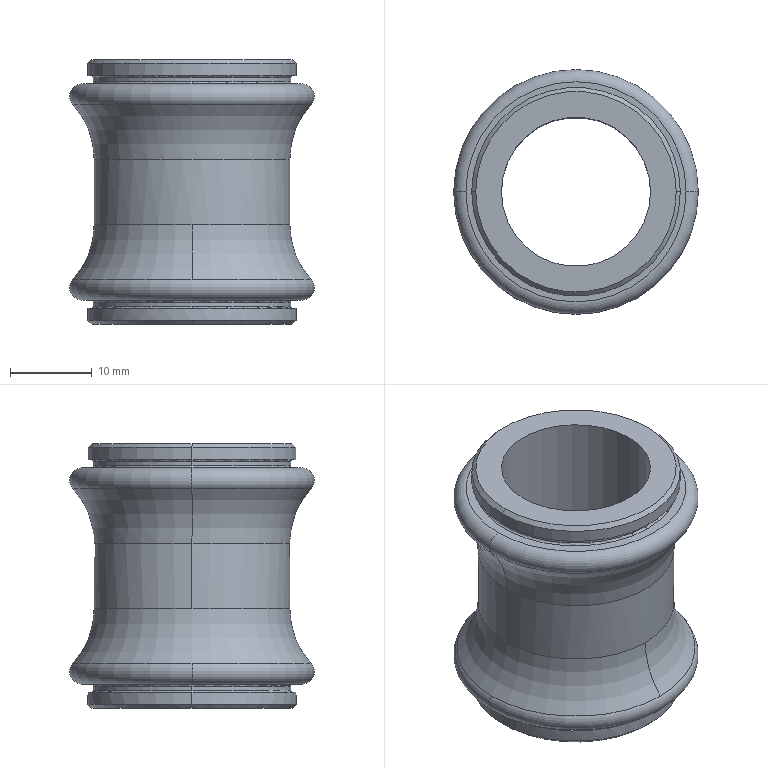Part | STEP file | _HSV08 -slide.... | 1 solid | 38 faces | box 30 x 30 x 32.5 mm | volume 8453 mm3 | torus 16 | cylinder 12 | plane 6 | cone 4 | commonest cylinder face diameters 24.2 x4 25.6 x4 18.3 x2 24 x2
STEP:
#1=CARTESIAN_POINT('',(-9.15,0.,0.));
#2=VERTEX_POINT('',#1);
#3=CARTESIAN_POINT('',(9.15,0.,0.));
#4=VERTEX_POINT('',#3);
#5=CARTESIAN_POINT('',(0.,0.,0.));
#6=DIRECTION('',(0.,0.,1.));
#7=DIRECTION('',(1.,0.,0.));
#8=AXIS2_PLACEMENT_3D('',#5,#6,#7);
#9=CIRCLE('',#8,9.15);
#10=EDGE_CURVE('',#2,#4,#9,.T.);
#11=ORIENTED_EDGE('',*,*,#10,.F.);
#12=CARTESIAN_POINT('',(-9.15,0.,32.5));
#13=VERTEX_POINT('',#12);
#14=CARTESIAN_POINT('',(-9.15,0.,0.));
#15=DIRECTION('',(0.,0.,1.));
#16=VECTOR('',#15,1000.);
#17=LINE('',#14,#16);
#18=EDGE_CURVE('',#2,#13,#17,.T.);
#19=ORIENTED_EDGE('',*,*,#18,.T.);
#20=CARTESIAN_POINT('',(9.15,0.,32.5));
#21=VERTEX_POINT('',#20);
#22=CARTESIAN_POINT('',(0.,0.,32.5));
#23=DIRECTION('',(0.,0.,-1.));
#24=DIRECTION('',(1.,0.,0.));
#25=AXIS2_PLACEMENT_3D('',#22,#23,#24);
#26=CIRCLE('',#25,9.15);
#27=EDGE_CURVE('',#21,#13,#26,.T.);
#28=ORIENTED_EDGE('',*,*,#27,.F.);
#29=CARTESIAN_POINT('',(9.15,0.,0.));
#30=DIRECTION('',(0.,0.,1.));
#31=VECTOR('',#30,1000.);
#32=LINE('',#29,#31);
#33=EDGE_CURVE('',#4,#21,#32,.T.);
#34=ORIENTED_EDGE('',*,*,#33,.F.);
#35=EDGE_LOOP('',(#11,#19,#28,#34));
#36=FACE_OUTER_BOUND('',#35,.T.);
#37=CARTESIAN_POINT('',(0.,0.,0.));
#38=DIRECTION('',(0.,0.,1.));
#39=DIRECTION('',(1.,0.,0.));
#40=AXIS2_PLACEMENT_3D('',#37,#38,#39);
#41=CYLINDRICAL_SURFACE('',#40,9.15);
#42=ADVANCED_FACE('',(#36),#41,.F.);
#43=CARTESIAN_POINT('',(0.,12.3,0.));
#44=VERTEX_POINT('',#43);
#45=CARTESIAN_POINT('',(0.,-12.3,0.));
#46=VERTEX_POINT('',#45);
#47=CARTESIAN_POINT('',(0.,0.,0.));
#48=DIRECTION('',(0.,0.,-1.));
#49=DIRECTION('',(0.,-1.,0.));
#50=AXIS2_PLACEMENT_3D('',#47,#48,#49);
#51=CIRCLE('',#50,12.3);
#52=EDGE_CURVE('',#44,#46,#51,.T.);
#53=ORIENTED_EDGE('',*,*,#52,.F.);
#54=CARTESIAN_POINT('',(0.,12.8,0.5));
#55=VERTEX_POINT('',#54);
#56=CARTESIAN_POINT('',(0.,12.8,0.5));
#57=DIRECTION('',(0.,0.7071,0.7071));
#58=VECTOR('',#57,1000.);
#59=LINE('',#56,#58);
#60=EDGE_CURVE('',#44,#55,#59,.T.);
#61=ORIENTED_EDGE('',*,*,#60,.T.);
#62=CARTESIAN_POINT('',(12.8,0.,0.5));
#63=VERTEX_POINT('',#62);
#64=CARTESIAN_POINT('',(0.,0.,0.5));
#65=DIRECTION('',(0.,0.,-1.));
#66=DIRECTION('',(1.,0.,0.));
#67=AXIS2_PLACEMENT_3D('',#64,#65,#66);
#68=CIRCLE('',#67,12.8);
#69=EDGE_CURVE('',#55,#63,#68,.T.);
#70=ORIENTED_EDGE('',*,*,#69,.T.);
#71=CARTESIAN_POINT('',(0.,-12.8,0.5));
#72=VERTEX_POINT('',#71);
#73=CARTESIAN_POINT('',(0.,0.,0.5));
#74=DIRECTION('',(0.,0.,-1.));
#75=DIRECTION('',(1.,0.,0.));
#76=AXIS2_PLACEMENT_3D('',#73,#74,#75);
#77=CIRCLE('',#76,12.8);
#78=EDGE_CURVE('',#63,#72,#77,.T.);
#79=ORIENTED_EDGE('',*,*,#78,.T.);
#80=CARTESIAN_POINT('',(0.,-12.8,0.5));
#81=DIRECTION('',(0.,-0.7071,0.7071));
#82=VECTOR('',#81,1000.);
#83=LINE('',#80,#82);
#84=EDGE_CURVE('',#46,#72,#83,.T.);
#85=ORIENTED_EDGE('',*,*,#84,.F.);
#86=EDGE_LOOP('',(#53,#61,#70,#79,#85));
#87=FACE_OUTER_BOUND('',#86,.T.);
#88=CARTESIAN_POINT('',(0.,0.,0.5));
#89=DIRECTION('',(0.,0.,1.));
#90=DIRECTION('',(0.,-1.,0.));
#91=AXIS2_PLACEMENT_3D('',#88,#89,#90);
#92=CONICAL_SURFACE('',#91,12.8,0.7854);
#93=ADVANCED_FACE('',(#87),#92,.T.);
#94=CARTESIAN_POINT('',(12.3,0.,32.5));
#95=VERTEX_POINT('',#94);
#96=CARTESIAN_POINT('',(-12.3,0.,32.5));
#97=VERTEX_POINT('',#96);
#98=CARTESIAN_POINT('',(0.,0.,32.5));
#99=DIRECTION('',(0.,0.,1.));
#100=DIRECTION('',(-1.,0.,0.));
#101=AXIS2_PLACEMENT_3D('',#98,#99,#100);
#102=CIRCLE('',#101,12.3);
#103=EDGE_CURVE('',#95,#97,#102,.T.);
#104=ORIENTED_EDGE('',*,*,#103,.F.);
#105=CARTESIAN_POINT('',(12.8,0.,32.));
#106=VERTEX_POINT('',#105);
#107=CARTESIAN_POINT('',(12.8,0.,32.));
#108=DIRECTION('',(0.7071,0.,-0.7071));
#109=VECTOR('',#108,1000.);
#110=LINE('',#107,#109);
#111=EDGE_CURVE('',#95,#106,#110,.T.);
#112=ORIENTED_EDGE('',*,*,#111,.T.);
#113=CARTESIAN_POINT('',(-12.8,0.,32.));
#114=VERTEX_POINT('',#113);
#115=CARTESIAN_POINT('',(0.,0.,32.));
#116=DIRECTION('',(0.,0.,1.));
#117=DIRECTION('',(-1.,0.,0.));
#118=AXIS2_PLACEMENT_3D('',#115,#116,#117);
#119=CIRCLE('',#118,12.8);
#120=EDGE_CURVE('',#106,#114,#119,.T.);
#121=ORIENTED_EDGE('',*,*,#120,.T.);
#122=CARTESIAN_POINT('',(-12.8,0.,32.));
#123=DIRECTION('',(-0.7071,0.,-0.7071));
#124=VECTOR('',#123,1000.);
#125=LINE('',#122,#124);
#126=EDGE_CURVE('',#97,#114,#125,.T.);
#127=ORIENTED_EDGE('',*,*,#126,.F.);
#128=EDGE_LOOP('',(#104,#112,#121,#127));
#129=FACE_OUTER_BOUND('',#128,.T.);
#130=CARTESIAN_POINT('',(0.,0.,32.));
#131=DIRECTION('',(0.,0.,-1.));
#132=DIRECTION('',(-1.,0.,0.));
#133=AXIS2_PLACEMENT_3D('',#130,#131,#132);
#134=CONICAL_SURFACE('',#133,12.8,0.7854);
#135=ADVANCED_FACE('',(#129),#134,.T.);
#136=CARTESIAN_POINT('',(-12.8,0.,0.5));
#137=VERTEX_POINT('',#136);
#138=CARTESIAN_POINT('',(0.,0.,0.5));
#139=DIRECTION('',(0.,0.,-1.));
#140=DIRECTION('',(1.,0.,0.));
#141=AXIS2_PLACEMENT_3D('',#138,#139,#140);
#142=CIRCLE('',#141,12.8);
#143=EDGE_CURVE('',#137,#55,#142,.T.);
#144=ORIENTED_EDGE('',*,*,#143,.F.);
#145=CARTESIAN_POINT('',(-12.8,0.,2.));
#146=VERTEX_POINT('',#145);
#147=CARTESIAN_POINT('',(-12.8,0.,0.));
#148=DIRECTION('',(0.,0.,1.));
#149=VECTOR('',#148,1000.);
#150=LINE('',#147,#149);
#151=EDGE_CURVE('',#137,#146,#150,.T.);
#152=ORIENTED_EDGE('',*,*,#151,.T.);
#153=CARTESIAN_POINT('',(12.8,0.,2.));
#154=VERTEX_POINT('',#153);
#155=CARTESIAN_POINT('',(0.,0.,2.));
#156=DIRECTION('',(0.,0.,-1.));
#157=DIRECTION('',(1.,0.,0.));
#158=AXIS2_PLACEMENT_3D('',#155,#156,#157);
#159=CIRCLE('',#158,12.8);
#160=EDGE_CURVE('',#146,#154,#159,.T.);
#161=ORIENTED_EDGE('',*,*,#160,.T.);
#162=CARTESIAN_POINT('',(12.8,0.,0.));
#163=DIRECTION('',(0.,0.,1.));
#164=VECTOR('',#163,1000.);
#165=LINE('',#162,#164);
#166=EDGE_CURVE('',#63,#154,#165,.T.);
#167=ORIENTED_EDGE('',*,*,#166,.F.);
#168=ORIENTED_EDGE('',*,*,#69,.F.);
#169=EDGE_LOOP('',(#144,#152,#161,#167,#168));
#170=FACE_OUTER_BOUND('',#169,.T.);
#171=CARTESIAN_POINT('',(0.,0.,0.));
#172=DIRECTION('',(0.,0.,1.));
#173=DIRECTION('',(1.,0.,0.));
#174=AXIS2_PLACEMENT_3D('',#171,#172,#173);
#175=CYLINDRICAL_SURFACE('',#174,12.8);
#176=ADVANCED_FACE('',(#170),#175,.T.);
#177=CARTESIAN_POINT('',(12.8,0.,30.5));
#178=VERTEX_POINT('',#177);
#179=CARTESIAN_POINT('',(-12.8,0.,30.5));
#180=VERTEX_POINT('',#179);
#181=CARTESIAN_POINT('',(0.,0.,30.5));
#182=DIRECTION('',(0.,0.,1.));
#183=DIRECTION('',(1.,0.,0.));
#184=AXIS2_PLACEMENT_3D('',#181,#182,#183);
#185=CIRCLE('',#184,12.8);
#186=EDGE_CURVE('',#178,#180,#185,.T.);
#187=ORIENTED_EDGE('',*,*,#186,.T.);
#188=CARTESIAN_POINT('',(-12.8,0.,0.));
#189=DIRECTION('',(0.,0.,1.));
#190=VECTOR('',#189,1000.);
#191=LINE('',#188,#190);
#192=EDGE_CURVE('',#180,#114,#191,.T.);
#193=ORIENTED_EDGE('',*,*,#192,.T.);
#194=ORIENTED_EDGE('',*,*,#120,.F.);
#195=CARTESIAN_POINT('',(12.8,0.,0.));
#196=DIRECTION('',(0.,0.,1.));
#197=VECTOR('',#196,1000.);
#198=LINE('',#195,#197);
#199=EDGE_CURVE('',#178,#106,#198,.T.);
#200=ORIENTED_EDGE('',*,*,#199,.F.);
#201=EDGE_LOOP('',(#187,#193,#194,#200));
#202=FACE_OUTER_BOUND('',#201,.T.);
#203=CARTESIAN_POINT('',(0.,0.,0.));
#204=DIRECTION('',(0.,0.,1.));
#205=DIRECTION('',(1.,0.,0.));
#206=AXIS2_PLACEMENT_3D('',#203,#204,#205);
#207=CYLINDRICAL_SURFACE('',#206,12.8);
#208=ADVANCED_FACE('',(#202),#207,.T.);
#209=CARTESIAN_POINT('',(0.,-12.35,2.));
#210=VERTEX_POINT('',#209);
#211=CARTESIAN_POINT('',(0.,12.35,2.));
#212=VERTEX_POINT('',#211);
#213=CARTESIAN_POINT('',(0.,0.,2.));
#214=DIRECTION('',(0.,0.,-1.));
#215=DIRECTION('',(0.,1.,0.));
#216=AXIS2_PLACEMENT_3D('',#213,#214,#215);
#217=CIRCLE('',#216,12.35);
#218=EDGE_CURVE('',#210,#212,#217,.T.);
#219=ORIENTED_EDGE('',*,*,#218,.F.);
#220=CARTESIAN_POINT('',(0.,-12.1,2.25));
#221=VERTEX_POINT('',#220);
#222=CARTESIAN_POINT('',(0.,-12.35,2.25));
#223=DIRECTION('',(1.,0.,0.));
#224=DIRECTION('',(0.,1.,0.));
#225=AXIS2_PLACEMENT_3D('',#222,#223,#224);
#226=CIRCLE('',#225,0.25);
#227=EDGE_CURVE('',#210,#221,#226,.T.);
#228=ORIENTED_EDGE('',*,*,#227,.T.);
#229=CARTESIAN_POINT('',(-12.1,0.,2.25));
#230=VERTEX_POINT('',#229);
#231=CARTESIAN_POINT('',(0.,0.,2.25));
#232=DIRECTION('',(0.,0.,1.));
#233=DIRECTION('',(1.,0.,0.));
#234=AXIS2_PLACEMENT_3D('',#231,#232,#233);
#235=CIRCLE('',#234,12.1);
#236=EDGE_CURVE('',#230,#221,#235,.T.);
#237=ORIENTED_EDGE('',*,*,#236,.F.);
#238=CARTESIAN_POINT('',(0.,12.1,2.25));
#239=VERTEX_POINT('',#238);
#240=CARTESIAN_POINT('',(0.,0.,2.25));
#241=DIRECTION('',(0.,0.,1.));
#242=DIRECTION('',(1.,0.,0.));
#243=AXIS2_PLACEMENT_3D('',#240,#241,#242);
#244=CIRCLE('',#243,12.1);
#245=EDGE_CURVE('',#239,#230,#244,.T.);
#246=ORIENTED_EDGE('',*,*,#245,.F.);
#247=CARTESIAN_POINT('',(0.,12.35,2.25));
#248=DIRECTION('',(-1.,0.,0.));
#249=DIRECTION('',(0.,0.,1.));
#250=AXIS2_PLACEMENT_3D('',#247,#248,#249);
#251=CIRCLE('',#250,0.25);
#252=EDGE_CURVE('',#212,#239,#251,.T.);
#253=ORIENTED_EDGE('',*,*,#252,.F.);
#254=EDGE_LOOP('',(#219,#228,#237,#246,#253));
#255=FACE_OUTER_BOUND('',#254,.T.);
#256=CARTESIAN_POINT('',(0.,0.,2.25));
#257=DIRECTION('',(0.,0.,-1.));
#258=DIRECTION('',(0.,1.,0.));
#259=AXIS2_PLACEMENT_3D('',#256,#257,#258);
#260=TOROIDAL_SURFACE('',#259,12.35,0.25);
#261=ADVANCED_FACE('',(#255),#260,.F.);
#262=CARTESIAN_POINT('',(0.,-12.1,30.25));
#263=VERTEX_POINT('',#262);
#264=CARTESIAN_POINT('',(-12.1,0.,30.25));
#265=VERTEX_POINT('',#264);
#266=CARTESIAN_POINT('',(0.,0.,30.25));
#267=DIRECTION('',(0.,0.,-1.));
#268=DIRECTION('',(-1.,0.,0.));
#269=AXIS2_PLACEMENT_3D('',#266,#267,#268);
#270=CIRCLE('',#269,12.1);
#271=EDGE_CURVE('',#263,#265,#270,.T.);
#272=ORIENTED_EDGE('',*,*,#271,.F.);
#273=CARTESIAN_POINT('',(0.,-12.35,30.5));
#274=VERTEX_POINT('',#273);
#275=CARTESIAN_POINT('',(0.,-12.35,30.25));
#276=DIRECTION('',(1.,0.,0.));
#277=DIRECTION('',(0.,1.,0.));
#278=AXIS2_PLACEMENT_3D('',#275,#276,#277);
#279=CIRCLE('',#278,0.25);
#280=EDGE_CURVE('',#263,#274,#279,.T.);
#281=ORIENTED_EDGE('',*,*,#280,.T.);
#282=CARTESIAN_POINT('',(0.,12.35,30.5));
#283=VERTEX_POINT('',#282);
#284=CARTESIAN_POINT('',(0.,0.,30.5));
#285=DIRECTION('',(0.,0.,1.));
#286=DIRECTION('',(0.,1.,0.));
#287=AXIS2_PLACEMENT_3D('',#284,#285,#286);
#288=CIRCLE('',#287,12.35);
#289=EDGE_CURVE('',#283,#274,#288,.T.);
#290=ORIENTED_EDGE('',*,*,#289,.F.);
#291=CARTESIAN_POINT('',(0.,12.1,30.25));
#292=VERTEX_POINT('',#291);
#293=CARTESIAN_POINT('',(0.,12.35,30.25));
#294=DIRECTION('',(-1.,0.,0.));
#295=DIRECTION('',(0.,0.,1.));
#296=AXIS2_PLACEMENT_3D('',#293,#294,#295);
#297=CIRCLE('',#296,0.25);
#298=EDGE_CURVE('',#292,#283,#297,.T.);
#299=ORIENTED_EDGE('',*,*,#298,.F.);
#300=CARTESIAN_POINT('',(0.,0.,30.25));
#301=DIRECTION('',(0.,0.,-1.));
#302=DIRECTION('',(-1.,0.,0.));
#303=AXIS2_PLACEMENT_3D('',#300,#301,#302);
#304=CIRCLE('',#303,12.1);
#305=EDGE_CURVE('',#265,#292,#304,.T.);
#306=ORIENTED_EDGE('',*,*,#305,.F.);
#307=EDGE_LOOP('',(#272,#281,#290,#299,#306));
#308=FACE_OUTER_BOUND('',#307,.T.);
#309=CARTESIAN_POINT('',(0.,0.,30.25));
#310=DIRECTION('',(0.,0.,-1.));
#311=DIRECTION('',(0.,1.,0.));
#312=AXIS2_PLACEMENT_3D('',#309,#310,#311);
#313=TOROIDAL_SURFACE('',#312,12.35,0.25);
#314=ADVANCED_FACE('',(#308),#313,.F.);
#315=CARTESIAN_POINT('',(12.1,0.,2.25));
#316=VERTEX_POINT('',#315);
#317=CARTESIAN_POINT('',(0.,0.,2.25));
#318=DIRECTION('',(0.,0.,1.));
#319=DIRECTION('',(1.,0.,0.));
#320=AXIS2_PLACEMENT_3D('',#317,#318,#319);
#321=CIRCLE('',#320,12.1);
#322=EDGE_CURVE('',#316,#239,#321,.T.);
#323=ORIENTED_EDGE('',*,*,#322,.T.);
#324=ORIENTED_EDGE('',*,*,#245,.T.);
#325=CARTESIAN_POINT('',(-12.1,0.,2.75));
#326=VERTEX_POINT('',#325);
#327=CARTESIAN_POINT('',(-12.1,0.,0.));
#328=DIRECTION('',(0.,0.,1.));
#329=VECTOR('',#328,1000.);
#330=LINE('',#327,#329);
#331=EDGE_CURVE('',#230,#326,#330,.T.);
#332=ORIENTED_EDGE('',*,*,#331,.T.);
#333=CARTESIAN_POINT('',(0.,12.1,2.75));
#334=VERTEX_POINT('',#333);
#335=CARTESIAN_POINT('',(0.,0.,2.75));
#336=DIRECTION('',(0.,0.,-1.));
#337=DIRECTION('',(1.,0.,0.));
#338=AXIS2_PLACEMENT_3D('',#335,#336,#337);
#339=CIRCLE('',#338,12.1);
#340=EDGE_CURVE('',#326,#334,#339,.T.);
#341=ORIENTED_EDGE('',*,*,#340,.T.);
#342=CARTESIAN_POINT('',(12.1,0.,2.75));
#343=VERTEX_POINT('',#342);
#344=CARTESIAN_POINT('',(0.,0.,2.75));
#345=DIRECTION('',(0.,0.,-1.));
#346=DIRECTION('',(1.,0.,0.));
#347=AXIS2_PLACEMENT_3D('',#344,#345,#346);
#348=CIRCLE('',#347,12.1);
#349=EDGE_CURVE('',#334,#343,#348,.T.);
#350=ORIENTED_EDGE('',*,*,#349,.T.);
#351=CARTESIAN_POINT('',(12.1,0.,0.));
#352=DIRECTION('',(0.,0.,1.));
#353=VECTOR('',#352,1000.);
#354=LINE('',#351,#353);
#355=EDGE_CURVE('',#316,#343,#354,.T.);
#356=ORIENTED_EDGE('',*,*,#355,.F.);
#357=EDGE_LOOP('',(#323,#324,#332,#341,#350,#356));
#358=FACE_OUTER_BOUND('',#357,.T.);
#359=CARTESIAN_POINT('',(0.,0.,0.));
#360=DIRECTION('',(0.,0.,1.));
#361=DIRECTION('',(1.,0.,0.));
#362=AXIS2_PLACEMENT_3D('',#359,#360,#361);
#363=CYLINDRICAL_SURFACE('',#362,12.1);
#364=ADVANCED_FACE('',(#358),#363,.T.);
#365=CARTESIAN_POINT('',(0.,12.1,29.75));
#366=VERTEX_POINT('',#365);
#367=CARTESIAN_POINT('',(-12.1,0.,29.75));
#368=VERTEX_POINT('',#367);
#369=CARTESIAN_POINT('',(0.,0.,29.75));
#370=DIRECTION('',(0.,0.,1.));
#371=DIRECTION('',(1.,0.,0.));
#372=AXIS2_PLACEMENT_3D('',#369,#370,#371);
#373=CIRCLE('',#372,12.1);
#374=EDGE_CURVE('',#366,#368,#373,.T.);
#375=ORIENTED_EDGE('',*,*,#374,.T.);
#376=CARTESIAN_POINT('',(-12.1,0.,0.));
#377=DIRECTION('',(0.,0.,1.));
#378=VECTOR('',#377,1000.);
#379=LINE('',#376,#378);
#380=EDGE_CURVE('',#368,#265,#379,.T.);
#381=ORIENTED_EDGE('',*,*,#380,.T.);
#382=ORIENTED_EDGE('',*,*,#305,.T.);
#383=CARTESIAN_POINT('',(12.1,0.,30.25));
#384=VERTEX_POINT('',#383);
#385=CARTESIAN_POINT('',(0.,0.,30.25));
#386=DIRECTION('',(0.,0.,-1.));
#387=DIRECTION('',(-1.,0.,0.));
#388=AXIS2_PLACEMENT_3D('',#385,#386,#387);
#389=CIRCLE('',#388,12.1);
#390=EDGE_CURVE('',#292,#384,#389,.T.);
#391=ORIENTED_EDGE('',*,*,#390,.T.);
#392=CARTESIAN_POINT('',(12.1,0.,29.75));
#393=VERTEX_POINT('',#392);
#394=CARTESIAN_POINT('',(12.1,0.,0.));
#395=DIRECTION('',(0.,0.,1.));
#396=VECTOR('',#395,1000.);
#397=LINE('',#394,#396);
#398=EDGE_CURVE('',#393,#384,#397,.T.);
#399=ORIENTED_EDGE('',*,*,#398,.F.);
#400=CARTESIAN_POINT('',(0.,0.,29.75));
#401=DIRECTION('',(0.,0.,1.));
#402=DIRECTION('',(1.,0.,0.));
#403=AXIS2_PLACEMENT_3D('',#400,#401,#402);
#404=CIRCLE('',#403,12.1);
#405=EDGE_CURVE('',#393,#366,#404,.T.);
#406=ORIENTED_EDGE('',*,*,#405,.T.);
#407=EDGE_LOOP('',(#375,#381,#382,#391,#399,#406));
#408=FACE_OUTER_BOUND('',#407,.T.);
#409=CARTESIAN_POINT('',(0.,0.,0.));
#410=DIRECTION('',(0.,0.,1.));
#411=DIRECTION('',(1.,0.,0.));
#412=AXIS2_PLACEMENT_3D('',#409,#410,#411);
#413=CYLINDRICAL_SURFACE('',#412,12.1);
#414=ADVANCED_FACE('',(#408),#413,.T.);
#415=CARTESIAN_POINT('',(0.,-12.1,2.75));
#416=VERTEX_POINT('',#415);
#417=CARTESIAN_POINT('',(0.,0.,2.75));
#418=DIRECTION('',(0.,0.,-1.));
#419=DIRECTION('',(1.,0.,0.));
#420=AXIS2_PLACEMENT_3D('',#417,#418,#419);
#421=CIRCLE('',#420,12.1);
#422=EDGE_CURVE('',#416,#326,#421,.T.);
#423=ORIENTED_EDGE('',*,*,#422,.F.);
#424=CARTESIAN_POINT('',(0.,-12.35,3.));
#425=VERTEX_POINT('',#424);
#426=CARTESIAN_POINT('',(0.,-12.35,2.75));
#427=DIRECTION('',(1.,0.,0.));
#428=DIRECTION('',(0.,1.,0.));
#429=AXIS2_PLACEMENT_3D('',#426,#427,#428);
#430=CIRCLE('',#429,0.25);
#431=EDGE_CURVE('',#416,#425,#430,.T.);
#432=ORIENTED_EDGE('',*,*,#431,.T.);
#433=CARTESIAN_POINT('',(0.,12.35,3.));
#434=VERTEX_POINT('',#433);
#435=CARTESIAN_POINT('',(0.,0.,3.));
#436=DIRECTION('',(0.,0.,1.));
#437=DIRECTION('',(0.,1.,0.));
#438=AXIS2_PLACEMENT_3D('',#435,#436,#437);
#439=CIRCLE('',#438,12.35);
#440=EDGE_CURVE('',#434,#425,#439,.T.);
#441=ORIENTED_EDGE('',*,*,#440,.F.);
#442=CARTESIAN_POINT('',(0.,12.35,2.75));
#443=DIRECTION('',(-1.,0.,0.));
#444=DIRECTION('',(0.,0.,1.));
#445=AXIS2_PLACEMENT_3D('',#442,#443,#444);
#446=CIRCLE('',#445,0.25);
#447=EDGE_CURVE('',#334,#434,#446,.T.);
#448=ORIENTED_EDGE('',*,*,#447,.F.);
#449=ORIENTED_EDGE('',*,*,#340,.F.);
#450=EDGE_LOOP('',(#423,#432,#441,#448,#449));
#451=FACE_OUTER_BOUND('',#450,.T.);
#452=CARTESIAN_POINT('',(0.,0.,2.75));
#453=DIRECTION('',(0.,0.,-1.));
#454=DIRECTION('',(0.,1.,0.));
#455=AXIS2_PLACEMENT_3D('',#452,#453,#454);
#456=TOROIDAL_SURFACE('',#455,12.35,0.25);
#457=ADVANCED_FACE('',(#451),#456,.F.);
#458=CARTESIAN_POINT('',(0.,-12.35,29.5));
#459=VERTEX_POINT('',#458);
#460=CARTESIAN_POINT('',(0.,12.35,29.5));
#461=VERTEX_POINT('',#460);
#462=CARTESIAN_POINT('',(0.,0.,29.5));
#463=DIRECTION('',(0.,0.,-1.));
#464=DIRECTION('',(0.,1.,0.));
#465=AXIS2_PLACEMENT_3D('',#462,#463,#464);
#466=CIRCLE('',#465,12.35);
#467=EDGE_CURVE('',#459,#461,#466,.T.);
#468=ORIENTED_EDGE('',*,*,#467,.F.);
#469=CARTESIAN_POINT('',(0.,-12.1,29.75));
#470=VERTEX_POINT('',#469);
#471=CARTESIAN_POINT('',(0.,-12.35,29.75));
#472=DIRECTION('',(1.,0.,0.));
#473=DIRECTION('',(0.,1.,0.));
#474=AXIS2_PLACEMENT_3D('',#471,#472,#473);
#475=CIRCLE('',#474,0.25);
#476=EDGE_CURVE('',#459,#470,#475,.T.);
#477=ORIENTED_EDGE('',*,*,#476,.T.);
#478=CARTESIAN_POINT('',(0.,0.,29.75));
#479=DIRECTION('',(0.,0.,1.));
#480=DIRECTION('',(1.,0.,0.));
#481=AXIS2_PLACEMENT_3D('',#478,#479,#480);
#482=CIRCLE('',#481,12.1);
#483=EDGE_CURVE('',#368,#470,#482,.T.);
#484=ORIENTED_EDGE('',*,*,#483,.F.);
#485=ORIENTED_EDGE('',*,*,#374,.F.);
#486=CARTESIAN_POINT('',(0.,12.35,29.75));
#487=DIRECTION('',(-1.,0.,0.));
#488=DIRECTION('',(0.,0.,1.));
#489=AXIS2_PLACEMENT_3D('',#486,#487,#488);
#490=CIRCLE('',#489,0.25);
#491=EDGE_CURVE('',#461,#366,#490,.T.);
#492=ORIENTED_EDGE('',*,*,#491,.F.);
#493=EDGE_LOOP('',(#468,#477,#484,#485,#492));
#494=FACE_OUTER_BOUND('',#493,.T.);
#495=CARTESIAN_POINT('',(0.,0.,29.75));
#496=DIRECTION('',(0.,0.,-1.));
#497=DIRECTION('',(0.,1.,0.));
#498=AXIS2_PLACEMENT_3D('',#495,#496,#497);
#499=TOROIDAL_SURFACE('',#498,12.35,0.25);
#500=ADVANCED_FACE('',(#494),#499,.F.);
#501=CARTESIAN_POINT('',(0.,14.609,5.51));
#502=VERTEX_POINT('',#501);
#503=CARTESIAN_POINT('',(14.609,0.,5.51));
#504=VERTEX_POINT('',#503);
#505=CARTESIAN_POINT('',(0.,0.,5.51));
#506=DIRECTION('',(0.,0.,-1.));
#507=DIRECTION('',(1.,0.,0.));
#508=AXIS2_PLACEMENT_3D('',#505,#506,#507);
#509=CIRCLE('',#508,14.609);
#510=EDGE_CURVE('',#502,#504,#509,.T.);
#511=ORIENTED_EDGE('',*,*,#510,.T.);
#512=CARTESIAN_POINT('',(13.5,0.,3.));
#513=VERTEX_POINT('',#512);
#514=CARTESIAN_POINT('',(13.5,0.,4.5));
#515=DIRECTION('',(0.,1.,0.));
#516=DIRECTION('',(-1.,0.,0.));
#517=AXIS2_PLACEMENT_3D('',#514,#515,#516);
#518=CIRCLE('',#517,1.5);
#519=EDGE_CURVE('',#504,#513,#518,.T.);
#520=ORIENTED_EDGE('',*,*,#519,.T.);
#521=CARTESIAN_POINT('',(-13.5,0.,3.));
#522=VERTEX_POINT('',#521);
#523=CARTESIAN_POINT('',(0.,0.,3.));
#524=DIRECTION('',(0.,0.,-1.));
#525=DIRECTION('',(-1.,0.,0.));
#526=AXIS2_PLACEMENT_3D('',#523,#524,#525);
#527=CIRCLE('',#526,13.5);
#528=EDGE_CURVE('',#522,#513,#527,.T.);
#529=ORIENTED_EDGE('',*,*,#528,.F.);
#530=CARTESIAN_POINT('',(-14.609,0.,5.51));
#531=VERTEX_POINT('',#530);
#532=CARTESIAN_POINT('',(-13.5,0.,4.5));
#533=DIRECTION('',(0.,-1.,0.));
#534=DIRECTION('',(0.,0.,-1.));
#535=AXIS2_PLACEMENT_3D('',#532,#533,#534);
#536=CIRCLE('',#535,1.5);
#537=EDGE_CURVE('',#531,#522,#536,.T.);
#538=ORIENTED_EDGE('',*,*,#537,.F.);
#539=CARTESIAN_POINT('',(0.,0.,5.51));
#540=DIRECTION('',(0.,0.,-1.));
#541=DIRECTION('',(1.,0.,0.));
#542=AXIS2_PLACEMENT_3D('',#539,#540,#541);
#543=CIRCLE('',#542,14.609);
#544=EDGE_CURVE('',#531,#502,#543,.T.);
#545=ORIENTED_EDGE('',*,*,#544,.T.);
#546=EDGE_LOOP('',(#511,#520,#529,#538,#545));
#547=FACE_OUTER_BOUND('',#546,.T.);
#548=CARTESIAN_POINT('',(0.,0.,4.5));
#549=DIRECTION('',(0.,0.,-1.));
#550=DIRECTION('',(-1.,0.,0.));
#551=AXIS2_PLACEMENT_3D('',#548,#549,#550);
#552=TOROIDAL_SURFACE('',#551,13.5,1.5);
#553=ADVANCED_FACE('',(#547),#552,.T.);
#554=CARTESIAN_POINT('',(13.5,0.,29.5));
#555=VERTEX_POINT('',#554);
#556=CARTESIAN_POINT('',(-13.5,0.,29.5));
#557=VERTEX_POINT('',#556);
#558=CARTESIAN_POINT('',(0.,0.,29.5));
#559=DIRECTION('',(0.,0.,1.));
#560=DIRECTION('',(-1.,0.,0.));
#561=AXIS2_PLACEMENT_3D('',#558,#559,#560);
#562=CIRCLE('',#561,13.5);
#563=EDGE_CURVE('',#555,#557,#562,.T.);
#564=ORIENTED_EDGE('',*,*,#563,.F.);
#565=CARTESIAN_POINT('',(14.609,0.,26.99));
#566=VERTEX_POINT('',#565);
#567=CARTESIAN_POINT('',(13.5,0.,28.));
#568=DIRECTION('',(0.,1.,0.));
#569=DIRECTION('',(-1.,0.,0.));
#570=AXIS2_PLACEMENT_3D('',#567,#568,#569);
#571=CIRCLE('',#570,1.5);
#572=EDGE_CURVE('',#555,#566,#571,.T.);
#573=ORIENTED_EDGE('',*,*,#572,.T.);
#574=CARTESIAN_POINT('',(-14.609,0.,26.99));
#575=VERTEX_POINT('',#574);
#576=CARTESIAN_POINT('',(0.,0.,26.99));
#577=DIRECTION('',(0.,0.,1.));
#578=DIRECTION('',(-1.,0.,0.));
#579=AXIS2_PLACEMENT_3D('',#576,#577,#578);
#580=CIRCLE('',#579,14.609);
#581=EDGE_CURVE('',#566,#575,#580,.T.);
#582=ORIENTED_EDGE('',*,*,#581,.T.);
#583=CARTESIAN_POINT('',(-13.5,0.,28.));
#584=DIRECTION('',(0.,-1.,0.));
#585=DIRECTION('',(0.,0.,-1.));
#586=AXIS2_PLACEMENT_3D('',#583,#584,#585);
#587=CIRCLE('',#586,1.5);
#588=EDGE_CURVE('',#557,#575,#587,.T.);
#589=ORIENTED_EDGE('',*,*,#588,.F.);
#590=EDGE_LOOP('',(#564,#573,#582,#589));
#591=FACE_OUTER_BOUND('',#590,.T.);
#592=CARTESIAN_POINT('',(0.,0.,28.));
#593=DIRECTION('',(0.,0.,-1.));
#594=DIRECTION('',(-1.,0.,0.));
#595=AXIS2_PLACEMENT_3D('',#592,#593,#594);
#596=TOROIDAL_SURFACE('',#595,13.5,1.5);
#597=ADVANCED_FACE('',(#591),#596,.T.);
#598=CARTESIAN_POINT('',(0.,-14.609,5.51));
#599=VERTEX_POINT('',#598);
#600=CARTESIAN_POINT('',(0.,0.,5.51));
#601=DIRECTION('',(0.,0.,-1.));
#602=DIRECTION('',(1.,0.,0.));
#603=AXIS2_PLACEMENT_3D('',#600,#601,#602);
#604=CIRCLE('',#603,14.609);
#605=EDGE_CURVE('',#599,#531,#604,.T.);
#606=ORIENTED_EDGE('',*,*,#605,.F.);
#607=CARTESIAN_POINT('',(0.,-12.,12.246));
#608=VERTEX_POINT('',#607);
#609=CARTESIAN_POINT('',(0.,-22.,12.246));
#610=DIRECTION('',(1.,0.,0.));
#611=DIRECTION('',(0.,1.,0.));
#612=AXIS2_PLACEMENT_3D('',#609,#610,#611);
#613=CIRCLE('',#612,10.);
#614=EDGE_CURVE('',#599,#608,#613,.T.);
#615=ORIENTED_EDGE('',*,*,#614,.T.);
#616=CARTESIAN_POINT('',(-12.,0.,12.246));
#617=VERTEX_POINT('',#616);
#618=CARTESIAN_POINT('',(0.,0.,12.246));
#619=DIRECTION('',(0.,0.,1.));
#620=DIRECTION('',(1.,0.,0.));
#621=AXIS2_PLACEMENT_3D('',#618,#619,#620);
#622=CIRCLE('',#621,12.);
#623=EDGE_CURVE('',#617,#608,#622,.T.);
#624=ORIENTED_EDGE('',*,*,#623,.F.);
#625=CARTESIAN_POINT('',(0.,12.,12.246));
#626=VERTEX_POINT('',#625);
#627=CARTESIAN_POINT('',(0.,0.,12.246));
#628=DIRECTION('',(0.,0.,1.));
#629=DIRECTION('',(1.,0.,0.));
#630=AXIS2_PLACEMENT_3D('',#627,#628,#629);
#631=CIRCLE('',#630,12.);
#632=EDGE_CURVE('',#626,#617,#631,.T.);
#633=ORIENTED_EDGE('',*,*,#632,.F.);
#634=CARTESIAN_POINT('',(0.,22.,12.246));
#635=DIRECTION('',(-1.,0.,0.));
#636=DIRECTION('',(0.,0.,1.));
#637=AXIS2_PLACEMENT_3D('',#634,#635,#636);
#638=CIRCLE('',#637,10.);
#639=EDGE_CURVE('',#502,#626,#638,.T.);
#640=ORIENTED_EDGE('',*,*,#639,.F.);
#641=ORIENTED_EDGE('',*,*,#544,.F.);
#642=EDGE_LOOP('',(#606,#615,#624,#633,#640,#641));
#643=FACE_OUTER_BOUND('',#642,.T.);
#644=CARTESIAN_POINT('',(0.,0.,12.246));
#645=DIRECTION('',(0.,0.,-1.));
#646=DIRECTION('',(0.,1.,0.));
#647=AXIS2_PLACEMENT_3D('',#644,#645,#646);
#648=TOROIDAL_SURFACE('',#647,22.,10.);
#649=ADVANCED_FACE('',(#643),#648,.F.);
#650=CARTESIAN_POINT('',(12.,0.,20.254));
#651=VERTEX_POINT('',#650);
#652=CARTESIAN_POINT('',(-12.,0.,20.254));
#653=VERTEX_POINT('',#652);
#654=CARTESIAN_POINT('',(0.,0.,20.254));
#655=DIRECTION('',(0.,0.,-1.));
#656=DIRECTION('',(-1.,0.,0.));
#657=AXIS2_PLACEMENT_3D('',#654,#655,#656);
#658=CIRCLE('',#657,12.);
#659=EDGE_CURVE('',#651,#653,#658,.T.);
#660=ORIENTED_EDGE('',*,*,#659,.F.);
#661=CARTESIAN_POINT('',(22.,0.,20.254));
#662=DIRECTION('',(0.,1.,0.));
#663=DIRECTION('',(-1.,0.,0.));
#664=AXIS2_PLACEMENT_3D('',#661,#662,#663);
#665=CIRCLE('',#664,10.);
#666=EDGE_CURVE('',#651,#566,#665,.T.);
#667=ORIENTED_EDGE('',*,*,#666,.T.);
#668=CARTESIAN_POINT('',(0.,0.,26.99));
#669=DIRECTION('',(0.,0.,1.));
#670=DIRECTION('',(-1.,0.,0.));
#671=AXIS2_PLACEMENT_3D('',#668,#669,#670);
#672=CIRCLE('',#671,14.609);
#673=EDGE_CURVE('',#575,#566,#672,.T.);
#674=ORIENTED_EDGE('',*,*,#673,.F.);
#675=CARTESIAN_POINT('',(-22.,0.,20.254));
#676=DIRECTION('',(0.,-1.,0.));
#677=DIRECTION('',(0.,0.,-1.));
#678=AXIS2_PLACEMENT_3D('',#675,#676,#677);
#679=CIRCLE('',#678,10.);
#680=EDGE_CURVE('',#653,#575,#679,.T.);
#681=ORIENTED_EDGE('',*,*,#680,.F.);
#682=EDGE_LOOP('',(#660,#667,#674,#681));
#683=FACE_OUTER_BOUND('',#682,.T.);
#684=CARTESIAN_POINT('',(0.,0.,20.254));
#685=DIRECTION('',(0.,0.,-1.));
#686=DIRECTION('',(-1.,0.,0.));
#687=AXIS2_PLACEMENT_3D('',#684,#685,#686);
#688=TOROIDAL_SURFACE('',#687,22.,10.);
#689=ADVANCED_FACE('',(#683),#688,.F.);
#690=CARTESIAN_POINT('',(12.,0.,12.246));
#691=VERTEX_POINT('',#690);
#692=CARTESIAN_POINT('',(0.,0.,12.246));
#693=DIRECTION('',(0.,0.,1.));
#694=DIRECTION('',(1.,0.,0.));
#695=AXIS2_PLACEMENT_3D('',#692,#693,#694);
#696=CIRCLE('',#695,12.);
#697=EDGE_CURVE('',#691,#626,#696,.T.);
#698=ORIENTED_EDGE('',*,*,#697,.T.);
#699=ORIENTED_EDGE('',*,*,#632,.T.);
#700=CARTESIAN_POINT('',(-12.,0.,0.));
#701=DIRECTION('',(0.,0.,1.));
#702=VECTOR('',#701,1000.);
#703=LINE('',#700,#702);
#704=EDGE_CURVE('',#617,#653,#703,.T.);
#705=ORIENTED_EDGE('',*,*,#704,.T.);
#706=CARTESIAN_POINT('',(0.,0.,20.254));
#707=DIRECTION('',(0.,0.,-1.));
#708=DIRECTION('',(-1.,0.,0.));
#709=AXIS2_PLACEMENT_3D('',#706,#707,#708);
#710=CIRCLE('',#709,12.);
#711=EDGE_CURVE('',#653,#651,#710,.T.);
#712=ORIENTED_EDGE('',*,*,#711,.T.);
#713=CARTESIAN_POINT('',(12.,0.,0.));
#714=DIRECTION('',(0.,0.,1.));
#715=VECTOR('',#714,1000.);
#716=LINE('',#713,#715);
#717=EDGE_CURVE('',#691,#651,#716,.T.);
#718=ORIENTED_EDGE('',*,*,#717,.F.);
#719=EDGE_LOOP('',(#698,#699,#705,#712,#718));
#720=FACE_OUTER_BOUND('',#719,.T.);
#721=CARTESIAN_POINT('',(0.,0.,0.));
#722=DIRECTION('',(0.,0.,1.));
#723=DIRECTION('',(1.,0.,0.));
#724=AXIS2_PLACEMENT_3D('',#721,#722,#723);
#725=CYLINDRICAL_SURFACE('',#724,12.);
#726=ADVANCED_FACE('',(#720),#725,.T.);
#727=ORIENTED_EDGE('',*,*,#18,.F.);
#728=CARTESIAN_POINT('',(0.,0.,0.));
#729=DIRECTION('',(0.,0.,1.));
#730=DIRECTION('',(1.,0.,0.));
#731=AXIS2_PLACEMENT_3D('',#728,#729,#730);
#732=CIRCLE('',#731,9.15);
#733=EDGE_CURVE('',#4,#2,#732,.T.);
#734=ORIENTED_EDGE('',*,*,#733,.F.);
#735=ORIENTED_EDGE('',*,*,#33,.T.);
#736=CARTESIAN_POINT('',(0.,0.,32.5));
#737=DIRECTION('',(0.,0.,-1.));
#738=DIRECTION('',(1.,0.,0.));
#739=AXIS2_PLACEMENT_3D('',#736,#737,#738);
#740=CIRCLE('',#739,9.15);
#741=EDGE_CURVE('',#13,#21,#740,.T.);
#742=ORIENTED_EDGE('',*,*,#741,.F.);
#743=EDGE_LOOP('',(#727,#734,#735,#742));
#744=FACE_OUTER_BOUND('',#743,.T.);
#745=CARTESIAN_POINT('',(0.,0.,0.));
#746=DIRECTION('',(0.,0.,1.));
#747=DIRECTION('',(1.,0.,0.));
#748=AXIS2_PLACEMENT_3D('',#745,#746,#747);
#749=CYLINDRICAL_SURFACE('',#748,9.15);
#750=ADVANCED_FACE('',(#744),#749,.F.);
#751=CARTESIAN_POINT('',(0.,0.,0.));
#752=DIRECTION('',(0.,0.,-1.));
#753=DIRECTION('',(0.,-1.,0.));
#754=AXIS2_PLACEMENT_3D('',#751,#752,#753);
#755=CIRCLE('',#754,12.3);
#756=EDGE_CURVE('',#46,#44,#755,.T.);
#757=ORIENTED_EDGE('',*,*,#756,.T.);
#758=ORIENTED_EDGE('',*,*,#52,.T.);
#759=EDGE_LOOP('',(#757,#758));
#760=FACE_OUTER_BOUND('',#759,.T.);
#761=ORIENTED_EDGE('',*,*,#733,.T.);
#762=ORIENTED_EDGE('',*,*,#10,.T.);
#763=EDGE_LOOP('',(#761,#762));
#764=FACE_BOUND('',#763,.T.);
#765=CARTESIAN_POINT('',(0.,9.15,0.));
#766=DIRECTION('',(0.,0.,-1.));
#767=DIRECTION('',(-1.,0.,0.));
#768=AXIS2_PLACEMENT_3D('',#765,#766,#767);
#769=PLANE('',#768);
#770=ADVANCED_FACE('',(#760,#764),#769,.T.);
#771=ORIENTED_EDGE('',*,*,#27,.T.);
#772=ORIENTED_EDGE('',*,*,#741,.T.);
#773=EDGE_LOOP('',(#771,#772));
#774=FACE_BOUND('',#773,.T.);
#775=CARTESIAN_POINT('',(0.,0.,32.5));
#776=DIRECTION('',(0.,0.,1.));
#777=DIRECTION('',(-1.,0.,0.));
#778=AXIS2_PLACEMENT_3D('',#775,#776,#777);
#779=CIRCLE('',#778,12.3);
#780=EDGE_CURVE('',#97,#95,#779,.T.);
#781=ORIENTED_EDGE('',*,*,#780,.T.);
#782=ORIENTED_EDGE('',*,*,#103,.T.);
#783=EDGE_LOOP('',(#781,#782));
#784=FACE_OUTER_BOUND('',#783,.T.);
#785=CARTESIAN_POINT('',(0.,12.3,32.5));
#786=DIRECTION('',(0.,0.,1.));
#787=DIRECTION('',(1.,0.,0.));
#788=AXIS2_PLACEMENT_3D('',#785,#786,#787);
#789=PLANE('',#788);
#790=ADVANCED_FACE('',(#774,#784),#789,.T.);
#791=ORIENTED_EDGE('',*,*,#60,.F.);
#792=ORIENTED_EDGE('',*,*,#756,.F.);
#793=ORIENTED_EDGE('',*,*,#84,.T.);
#794=CARTESIAN_POINT('',(0.,0.,0.5));
#795=DIRECTION('',(0.,0.,-1.));
#796=DIRECTION('',(1.,0.,0.));
#797=AXIS2_PLACEMENT_3D('',#794,#795,#796);
#798=CIRCLE('',#797,12.8);
#799=EDGE_CURVE('',#72,#137,#798,.T.);
#800=ORIENTED_EDGE('',*,*,#799,.T.);
#801=ORIENTED_EDGE('',*,*,#143,.T.);
#802=EDGE_LOOP('',(#791,#792,#793,#800,#801));
#803=FACE_OUTER_BOUND('',#802,.T.);
#804=CARTESIAN_POINT('',(0.,0.,0.5));
#805=DIRECTION('',(0.,0.,1.));
#806=DIRECTION('',(0.,-1.,0.));
#807=AXIS2_PLACEMENT_3D('',#804,#805,#806);
#808=CONICAL_SURFACE('',#807,12.8,0.7854);
#809=ADVANCED_FACE('',(#803),#808,.T.);
#810=ORIENTED_EDGE('',*,*,#111,.F.);
#811=ORIENTED_EDGE('',*,*,#780,.F.);
#812=ORIENTED_EDGE('',*,*,#126,.T.);
#813=CARTESIAN_POINT('',(0.,0.,32.));
#814=DIRECTION('',(0.,0.,1.));
#815=DIRECTION('',(-1.,0.,0.));
#816=AXIS2_PLACEMENT_3D('',#813,#814,#815);
#817=CIRCLE('',#816,12.8);
#818=EDGE_CURVE('',#114,#106,#817,.T.);
#819=ORIENTED_EDGE('',*,*,#818,.T.);
#820=EDGE_LOOP('',(#810,#811,#812,#819));
#821=FACE_OUTER_BOUND('',#820,.T.);
#822=CARTESIAN_POINT('',(0.,0.,32.));
#823=DIRECTION('',(0.,0.,-1.));
#824=DIRECTION('',(-1.,0.,0.));
#825=AXIS2_PLACEMENT_3D('',#822,#823,#824);
#826=CONICAL_SURFACE('',#825,12.8,0.7854);
#827=ADVANCED_FACE('',(#821),#826,.T.);
#828=ORIENTED_EDGE('',*,*,#151,.F.);
#829=ORIENTED_EDGE('',*,*,#799,.F.);
#830=ORIENTED_EDGE('',*,*,#78,.F.);
#831=ORIENTED_EDGE('',*,*,#166,.T.);
#832=CARTESIAN_POINT('',(0.,0.,2.));
#833=DIRECTION('',(0.,0.,-1.));
#834=DIRECTION('',(1.,0.,0.));
#835=AXIS2_PLACEMENT_3D('',#832,#833,#834);
#836=CIRCLE('',#835,12.8);
#837=EDGE_CURVE('',#154,#146,#836,.T.);
#838=ORIENTED_EDGE('',*,*,#837,.T.);
#839=EDGE_LOOP('',(#828,#829,#830,#831,#838));
#840=FACE_OUTER_BOUND('',#839,.T.);
#841=CARTESIAN_POINT('',(0.,0.,0.));
#842=DIRECTION('',(0.,0.,1.));
#843=DIRECTION('',(1.,0.,0.));
#844=AXIS2_PLACEMENT_3D('',#841,#842,#843);
#845=CYLINDRICAL_SURFACE('',#844,12.8);
#846=ADVANCED_FACE('',(#840),#845,.T.);
#847=ORIENTED_EDGE('',*,*,#192,.F.);
#848=CARTESIAN_POINT('',(0.,0.,30.5));
#849=DIRECTION('',(0.,0.,1.));
#850=DIRECTION('',(1.,0.,0.));
#851=AXIS2_PLACEMENT_3D('',#848,#849,#850);
#852=CIRCLE('',#851,12.8);
#853=EDGE_CURVE('',#180,#178,#852,.T.);
#854=ORIENTED_EDGE('',*,*,#853,.T.);
#855=ORIENTED_EDGE('',*,*,#199,.T.);
#856=ORIENTED_EDGE('',*,*,#818,.F.);
#857=EDGE_LOOP('',(#847,#854,#855,#856));
#858=FACE_OUTER_BOUND('',#857,.T.);
#859=CARTESIAN_POINT('',(0.,0.,0.));
#860=DIRECTION('',(0.,0.,1.));
#861=DIRECTION('',(1.,0.,0.));
#862=AXIS2_PLACEMENT_3D('',#859,#860,#861);
#863=CYLINDRICAL_SURFACE('',#862,12.8);
#864=ADVANCED_FACE('',(#858),#863,.T.);
#865=CARTESIAN_POINT('',(0.,0.,2.));
#866=DIRECTION('',(0.,0.,-1.));
#867=DIRECTION('',(0.,1.,0.));
#868=AXIS2_PLACEMENT_3D('',#865,#866,#867);
#869=CIRCLE('',#868,12.35);
#870=EDGE_CURVE('',#212,#210,#869,.T.);
#871=ORIENTED_EDGE('',*,*,#870,.T.);
#872=ORIENTED_EDGE('',*,*,#218,.T.);
#873=EDGE_LOOP('',(#871,#872));
#874=FACE_BOUND('',#873,.T.);
#875=ORIENTED_EDGE('',*,*,#837,.F.);
#876=ORIENTED_EDGE('',*,*,#160,.F.);
#877=EDGE_LOOP('',(#875,#876));
#878=FACE_OUTER_BOUND('',#877,.T.);
#879=CARTESIAN_POINT('',(0.,12.8,2.));
#880=DIRECTION('',(0.,0.,1.));
#881=DIRECTION('',(1.,0.,0.));
#882=AXIS2_PLACEMENT_3D('',#879,#880,#881);
#883=PLANE('',#882);
#884=ADVANCED_FACE('',(#874,#878),#883,.T.);
#885=ORIENTED_EDGE('',*,*,#186,.F.);
#886=ORIENTED_EDGE('',*,*,#853,.F.);
#887=EDGE_LOOP('',(#885,#886));
#888=FACE_OUTER_BOUND('',#887,.T.);
#889=ORIENTED_EDGE('',*,*,#289,.T.);
#890=CARTESIAN_POINT('',(0.,0.,30.5));
#891=DIRECTION('',(0.,0.,1.));
#892=DIRECTION('',(0.,1.,0.));
#893=AXIS2_PLACEMENT_3D('',#890,#891,#892);
#894=CIRCLE('',#893,12.35);
#895=EDGE_CURVE('',#274,#283,#894,.T.);
#896=ORIENTED_EDGE('',*,*,#895,.T.);
#897=EDGE_LOOP('',(#889,#896));
#898=FACE_BOUND('',#897,.T.);
#899=CARTESIAN_POINT('',(0.,12.35,30.5));
#900=DIRECTION('',(0.,0.,-1.));
#901=DIRECTION('',(-1.,0.,0.));
#902=AXIS2_PLACEMENT_3D('',#899,#900,#901);
#903=PLANE('',#902);
#904=ADVANCED_FACE('',(#888,#898),#903,.T.);
#905=ORIENTED_EDGE('',*,*,#227,.F.);
#906=ORIENTED_EDGE('',*,*,#870,.F.);
#907=ORIENTED_EDGE('',*,*,#252,.T.);
#908=ORIENTED_EDGE('',*,*,#322,.F.);
#909=CARTESIAN_POINT('',(0.,0.,2.25));
#910=DIRECTION('',(0.,0.,1.));
#911=DIRECTION('',(1.,0.,0.));
#912=AXIS2_PLACEMENT_3D('',#909,#910,#911);
#913=CIRCLE('',#912,12.1);
#914=EDGE_CURVE('',#221,#316,#913,.T.);
#915=ORIENTED_EDGE('',*,*,#914,.F.);
#916=EDGE_LOOP('',(#905,#906,#907,#908,#915));
#917=FACE_OUTER_BOUND('',#916,.T.);
#918=CARTESIAN_POINT('',(0.,0.,2.25));
#919=DIRECTION('',(0.,0.,-1.));
#920=DIRECTION('',(0.,1.,0.));
#921=AXIS2_PLACEMENT_3D('',#918,#919,#920);
#922=TOROIDAL_SURFACE('',#921,12.35,0.25);
#923=ADVANCED_FACE('',(#917),#922,.F.);
#924=ORIENTED_EDGE('',*,*,#280,.F.);
#925=CARTESIAN_POINT('',(0.,0.,30.25));
#926=DIRECTION('',(0.,0.,-1.));
#927=DIRECTION('',(-1.,0.,0.));
#928=AXIS2_PLACEMENT_3D('',#925,#926,#927);
#929=CIRCLE('',#928,12.1);
#930=EDGE_CURVE('',#384,#263,#929,.T.);
#931=ORIENTED_EDGE('',*,*,#930,.F.);
#932=ORIENTED_EDGE('',*,*,#390,.F.);
#933=ORIENTED_EDGE('',*,*,#298,.T.);
#934=ORIENTED_EDGE('',*,*,#895,.F.);
#935=EDGE_LOOP('',(#924,#931,#932,#933,#934));
#936=FACE_OUTER_BOUND('',#935,.T.);
#937=CARTESIAN_POINT('',(0.,0.,30.25));
#938=DIRECTION('',(0.,0.,-1.));
#939=DIRECTION('',(0.,1.,0.));
#940=AXIS2_PLACEMENT_3D('',#937,#938,#939);
#941=TOROIDAL_SURFACE('',#940,12.35,0.25);
#942=ADVANCED_FACE('',(#936),#941,.F.);
#943=ORIENTED_EDGE('',*,*,#331,.F.);
#944=ORIENTED_EDGE('',*,*,#236,.T.);
#945=ORIENTED_EDGE('',*,*,#914,.T.);
#946=ORIENTED_EDGE('',*,*,#355,.T.);
#947=CARTESIAN_POINT('',(0.,0.,2.75));
#948=DIRECTION('',(0.,0.,-1.));
#949=DIRECTION('',(1.,0.,0.));
#950=AXIS2_PLACEMENT_3D('',#947,#948,#949);
#951=CIRCLE('',#950,12.1);
#952=EDGE_CURVE('',#343,#416,#951,.T.);
#953=ORIENTED_EDGE('',*,*,#952,.T.);
#954=ORIENTED_EDGE('',*,*,#422,.T.);
#955=EDGE_LOOP('',(#943,#944,#945,#946,#953,#954));
#956=FACE_OUTER_BOUND('',#955,.T.);
#957=CARTESIAN_POINT('',(0.,0.,0.));
#958=DIRECTION('',(0.,0.,1.));
#959=DIRECTION('',(1.,0.,0.));
#960=AXIS2_PLACEMENT_3D('',#957,#958,#959);
#961=CYLINDRICAL_SURFACE('',#960,12.1);
#962=ADVANCED_FACE('',(#956),#961,.T.);
#963=ORIENTED_EDGE('',*,*,#380,.F.);
#964=ORIENTED_EDGE('',*,*,#483,.T.);
#965=CARTESIAN_POINT('',(0.,0.,29.75));
#966=DIRECTION('',(0.,0.,1.));
#967=DIRECTION('',(1.,0.,0.));
#968=AXIS2_PLACEMENT_3D('',#965,#966,#967);
#969=CIRCLE('',#968,12.1);
#970=EDGE_CURVE('',#470,#393,#969,.T.);
#971=ORIENTED_EDGE('',*,*,#970,.T.);
#972=ORIENTED_EDGE('',*,*,#398,.T.);
#973=ORIENTED_EDGE('',*,*,#930,.T.);
#974=ORIENTED_EDGE('',*,*,#271,.T.);
#975=EDGE_LOOP('',(#963,#964,#971,#972,#973,#974));
#976=FACE_OUTER_BOUND('',#975,.T.);
#977=CARTESIAN_POINT('',(0.,0.,0.));
#978=DIRECTION('',(0.,0.,1.));
#979=DIRECTION('',(1.,0.,0.));
#980=AXIS2_PLACEMENT_3D('',#977,#978,#979);
#981=CYLINDRICAL_SURFACE('',#980,12.1);
#982=ADVANCED_FACE('',(#976),#981,.T.);
#983=ORIENTED_EDGE('',*,*,#431,.F.);
#984=ORIENTED_EDGE('',*,*,#952,.F.);
#985=ORIENTED_EDGE('',*,*,#349,.F.);
#986=ORIENTED_EDGE('',*,*,#447,.T.);
#987=CARTESIAN_POINT('',(0.,0.,3.));
#988=DIRECTION('',(0.,0.,1.));
#989=DIRECTION('',(0.,1.,0.));
#990=AXIS2_PLACEMENT_3D('',#987,#988,#989);
#991=CIRCLE('',#990,12.35);
#992=EDGE_CURVE('',#425,#434,#991,.T.);
#993=ORIENTED_EDGE('',*,*,#992,.F.);
#994=EDGE_LOOP('',(#983,#984,#985,#986,#993));
#995=FACE_OUTER_BOUND('',#994,.T.);
#996=CARTESIAN_POINT('',(0.,0.,2.75));
#997=DIRECTION('',(0.,0.,-1.));
#998=DIRECTION('',(0.,1.,0.));
#999=AXIS2_PLACEMENT_3D('',#996,#997,#998);
#1000=TOROIDAL_SURFACE('',#999,12.35,0.25);
#1001=ADVANCED_FACE('',(#995),#1000,.F.);
#1002=ORIENTED_EDGE('',*,*,#476,.F.);
#1003=CARTESIAN_POINT('',(0.,0.,29.5));
#1004=DIRECTION('',(0.,0.,-1.));
#1005=DIRECTION('',(0.,1.,0.));
#1006=AXIS2_PLACEMENT_3D('',#1003,#1004,#1005);
#1007=CIRCLE('',#1006,12.35);
#1008=EDGE_CURVE('',#461,#459,#1007,.T.);
#1009=ORIENTED_EDGE('',*,*,#1008,.F.);
#1010=ORIENTED_EDGE('',*,*,#491,.T.);
#1011=ORIENTED_EDGE('',*,*,#405,.F.);
#1012=ORIENTED_EDGE('',*,*,#970,.F.);
#1013=EDGE_LOOP('',(#1002,#1009,#1010,#1011,#1012));
#1014=FACE_OUTER_BOUND('',#1013,.T.);
#1015=CARTESIAN_POINT('',(0.,0.,29.75));
#1016=DIRECTION('',(0.,0.,-1.));
#1017=DIRECTION('',(0.,1.,0.));
#1018=AXIS2_PLACEMENT_3D('',#1015,#1016,#1017);
#1019=TOROIDAL_SURFACE('',#1018,12.35,0.25);
#1020=ADVANCED_FACE('',(#1014),#1019,.F.);
#1021=ORIENTED_EDGE('',*,*,#528,.T.);
#1022=CARTESIAN_POINT('',(0.,0.,3.));
#1023=DIRECTION('',(0.,0.,-1.));
#1024=DIRECTION('',(-1.,0.,0.));
#1025=AXIS2_PLACEMENT_3D('',#1022,#1023,#1024);
#1026=CIRCLE('',#1025,13.5);
#1027=EDGE_CURVE('',#513,#522,#1026,.T.);
#1028=ORIENTED_EDGE('',*,*,#1027,.T.);
#1029=EDGE_LOOP('',(#1021,#1028));
#1030=FACE_OUTER_BOUND('',#1029,.T.);
#1031=ORIENTED_EDGE('',*,*,#440,.T.);
#1032=ORIENTED_EDGE('',*,*,#992,.T.);
#1033=EDGE_LOOP('',(#1031,#1032));
#1034=FACE_BOUND('',#1033,.T.);
#1035=CARTESIAN_POINT('',(0.,12.35,3.));
#1036=DIRECTION('',(0.,0.,-1.));
#1037=DIRECTION('',(-1.,0.,0.));
#1038=AXIS2_PLACEMENT_3D('',#1035,#1036,#1037);
#1039=PLANE('',#1038);
#1040=ADVANCED_FACE('',(#1030,#1034),#1039,.T.);
#1041=ORIENTED_EDGE('',*,*,#1008,.T.);
#1042=ORIENTED_EDGE('',*,*,#467,.T.);
#1043=EDGE_LOOP('',(#1041,#1042));
#1044=FACE_BOUND('',#1043,.T.);
#1045=CARTESIAN_POINT('',(0.,0.,29.5));
#1046=DIRECTION('',(0.,0.,1.));
#1047=DIRECTION('',(-1.,0.,0.));
#1048=AXIS2_PLACEMENT_3D('',#1045,#1046,#1047);
#1049=CIRCLE('',#1048,13.5);
#1050=EDGE_CURVE('',#557,#555,#1049,.T.);
#1051=ORIENTED_EDGE('',*,*,#1050,.T.);
#1052=ORIENTED_EDGE('',*,*,#563,.T.);
#1053=EDGE_LOOP('',(#1051,#1052));
#1054=FACE_OUTER_BOUND('',#1053,.T.);
#1055=CARTESIAN_POINT('',(0.,13.5,29.5));
#1056=DIRECTION('',(0.,0.,1.));
#1057=DIRECTION('',(1.,0.,0.));
#1058=AXIS2_PLACEMENT_3D('',#1055,#1056,#1057);
#1059=PLANE('',#1058);
#1060=ADVANCED_FACE('',(#1044,#1054),#1059,.T.);
#1061=ORIENTED_EDGE('',*,*,#519,.F.);
#1062=CARTESIAN_POINT('',(0.,0.,5.51));
#1063=DIRECTION('',(0.,0.,-1.));
#1064=DIRECTION('',(1.,0.,0.));
#1065=AXIS2_PLACEMENT_3D('',#1062,#1063,#1064);
#1066=CIRCLE('',#1065,14.609);
#1067=EDGE_CURVE('',#504,#599,#1066,.T.);
#1068=ORIENTED_EDGE('',*,*,#1067,.T.);
#1069=ORIENTED_EDGE('',*,*,#605,.T.);
#1070=ORIENTED_EDGE('',*,*,#537,.T.);
#1071=ORIENTED_EDGE('',*,*,#1027,.F.);
#1072=EDGE_LOOP('',(#1061,#1068,#1069,#1070,#1071));
#1073=FACE_OUTER_BOUND('',#1072,.T.);
#1074=CARTESIAN_POINT('',(0.,0.,4.5));
#1075=DIRECTION('',(0.,0.,-1.));
#1076=DIRECTION('',(-1.,0.,0.));
#1077=AXIS2_PLACEMENT_3D('',#1074,#1075,#1076);
#1078=TOROIDAL_SURFACE('',#1077,13.5,1.5);
#1079=ADVANCED_FACE('',(#1073),#1078,.T.);
#1080=ORIENTED_EDGE('',*,*,#572,.F.);
#1081=ORIENTED_EDGE('',*,*,#1050,.F.);
#1082=ORIENTED_EDGE('',*,*,#588,.T.);
#1083=ORIENTED_EDGE('',*,*,#673,.T.);
#1084=EDGE_LOOP('',(#1080,#1081,#1082,#1083));
#1085=FACE_OUTER_BOUND('',#1084,.T.);
#1086=CARTESIAN_POINT('',(0.,0.,28.));
#1087=DIRECTION('',(0.,0.,-1.));
#1088=DIRECTION('',(-1.,0.,0.));
#1089=AXIS2_PLACEMENT_3D('',#1086,#1087,#1088);
#1090=TOROIDAL_SURFACE('',#1089,13.5,1.5);
#1091=ADVANCED_FACE('',(#1085),#1090,.T.);
#1092=ORIENTED_EDGE('',*,*,#614,.F.);
#1093=ORIENTED_EDGE('',*,*,#1067,.F.);
#1094=ORIENTED_EDGE('',*,*,#510,.F.);
#1095=ORIENTED_EDGE('',*,*,#639,.T.);
#1096=ORIENTED_EDGE('',*,*,#697,.F.);
#1097=CARTESIAN_POINT('',(0.,0.,12.246));
#1098=DIRECTION('',(0.,0.,1.));
#1099=DIRECTION('',(1.,0.,0.));
#1100=AXIS2_PLACEMENT_3D('',#1097,#1098,#1099);
#1101=CIRCLE('',#1100,12.);
#1102=EDGE_CURVE('',#608,#691,#1101,.T.);
#1103=ORIENTED_EDGE('',*,*,#1102,.F.);
#1104=EDGE_LOOP('',(#1092,#1093,#1094,#1095,#1096,#1103));
#1105=FACE_OUTER_BOUND('',#1104,.T.);
#1106=CARTESIAN_POINT('',(0.,0.,12.246));
#1107=DIRECTION('',(0.,0.,-1.));
#1108=DIRECTION('',(0.,1.,0.));
#1109=AXIS2_PLACEMENT_3D('',#1106,#1107,#1108);
#1110=TOROIDAL_SURFACE('',#1109,22.,10.);
#1111=ADVANCED_FACE('',(#1105),#1110,.F.);
#1112=ORIENTED_EDGE('',*,*,#666,.F.);
#1113=ORIENTED_EDGE('',*,*,#711,.F.);
#1114=ORIENTED_EDGE('',*,*,#680,.T.);
#1115=ORIENTED_EDGE('',*,*,#581,.F.);
#1116=EDGE_LOOP('',(#1112,#1113,#1114,#1115));
#1117=FACE_OUTER_BOUND('',#1116,.T.);
#1118=CARTESIAN_POINT('',(0.,0.,20.254));
#1119=DIRECTION('',(0.,0.,-1.));
#1120=DIRECTION('',(-1.,0.,0.));
#1121=AXIS2_PLACEMENT_3D('',#1118,#1119,#1120);
#1122=TOROIDAL_SURFACE('',#1121,22.,10.);
#1123=ADVANCED_FACE('',(#1117),#1122,.F.);
#1124=ORIENTED_EDGE('',*,*,#704,.F.);
#1125=ORIENTED_EDGE('',*,*,#623,.T.);
#1126=ORIENTED_EDGE('',*,*,#1102,.T.);
#1127=ORIENTED_EDGE('',*,*,#717,.T.);
#1128=ORIENTED_EDGE('',*,*,#659,.T.);
#1129=EDGE_LOOP('',(#1124,#1125,#1126,#1127,#1128));
#1130=FACE_OUTER_BOUND('',#1129,.T.);
#1131=CARTESIAN_POINT('',(0.,0.,0.));
#1132=DIRECTION('',(0.,0.,1.));
#1133=DIRECTION('',(1.,0.,0.));
#1134=AXIS2_PLACEMENT_3D('',#1131,#1132,#1133);
#1135=CYLINDRICAL_SURFACE('',#1134,12.);
#1136=ADVANCED_FACE('',(#1130),#1135,.T.);
#1137=CLOSED_SHELL('',(#42,#93,#135,#176,#208,#261,#314,#364,#414,#457,#500,#553,#597,#649,#689,#726,#750,#770,#790,#809,#827,#846,#864,#884,#904,#923,#942,#962,#982,#1001,#1020,#1040,#1060,#1079,#1091,#1111,#1123,#1136));
#1138=MANIFOLD_SOLID_BREP('',#1137);
#1139=CARTESIAN_POINT('',(0.,0.,0.));
#1140=DIRECTION('',(0.,0.,1.));
#1141=DIRECTION('',(1.,0.,0.));
#1142=AXIS2_PLACEMENT_3D('',#1139,#1140,#1141);
#1143=(LENGTH_UNIT()NAMED_UNIT(*)SI_UNIT(.MILLI.,.METRE.));
#1144=UNCERTAINTY_MEASURE_WITH_UNIT(LENGTH_MEASURE(0.00001),#1143,'','');
#1145=(NAMED_UNIT(*)PLANE_ANGLE_UNIT()SI_UNIT($,.RADIAN.));
#1146=(NAMED_UNIT(*)SI_UNIT($,.STERADIAN.)SOLID_ANGLE_UNIT());
#1147=(GEOMETRIC_REPRESENTATION_CONTEXT(3)GLOBAL_UNCERTAINTY_ASSIGNED_CONTEXT((#1144))GLOBAL_UNIT_ASSIGNED_CONTEXT((#1143,#1145,#1146))REPRESENTATION_CONTEXT('',''));
#1148=ADVANCED_BREP_SHAPE_REPRESENTATION('',(#1138,#1142),#1147);